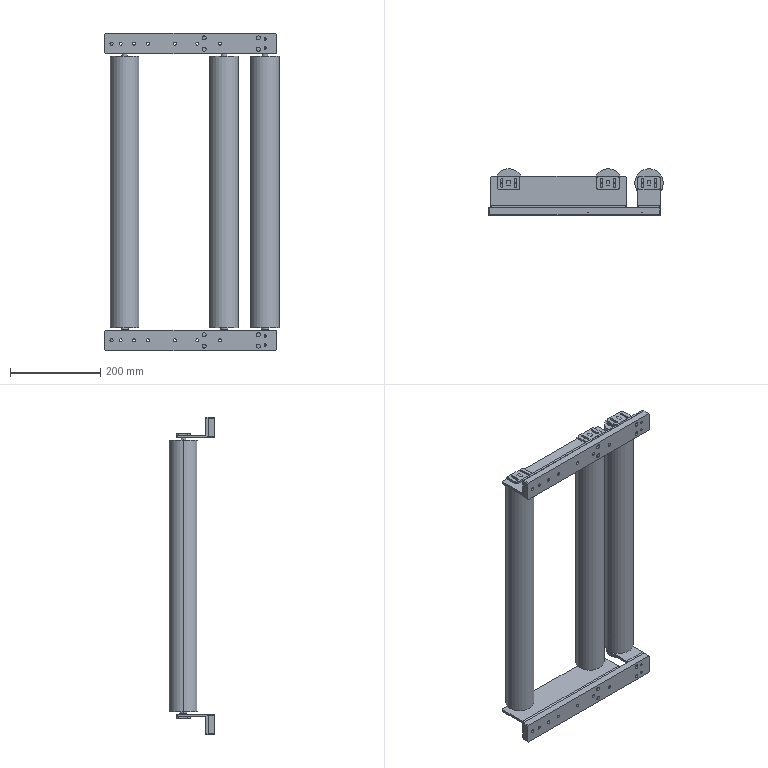Part | SolidWorks | 15 solids | 441 faces | box 386.25 x 101.5 x 702 mm | volume 6495090 mm3 | plane 221 | cylinder 220 | commonest cylinder face diameters 4.5 x36 12 x30 6.8 x28 3.3 x24 10 x24 9 x16